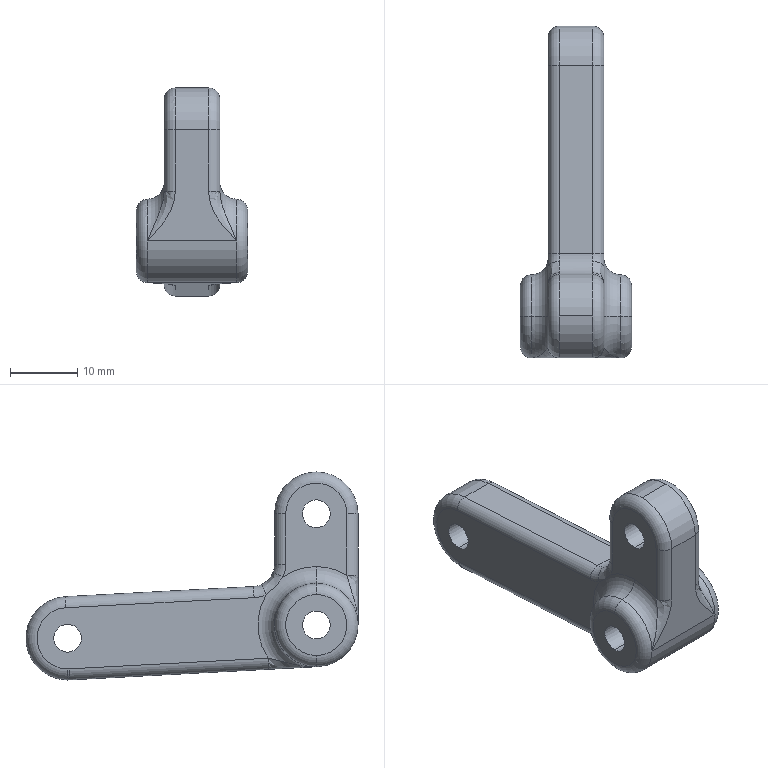Part | SolidWorks | features Fillet 3, ICE 3, 3DProfileFeature 2, Extrusion 1, Scale 1 | 1 solid | 55 faces | box 16.51 x 49.289 x 30.864 mm | volume 6856 mm3 | torus 20 | cylinder 19 | plane 10 | spline 6 | commonest cylinder face diameters 3.302 x8 4.127 x4 12.383 x4 4.128 x2 6.604 x1